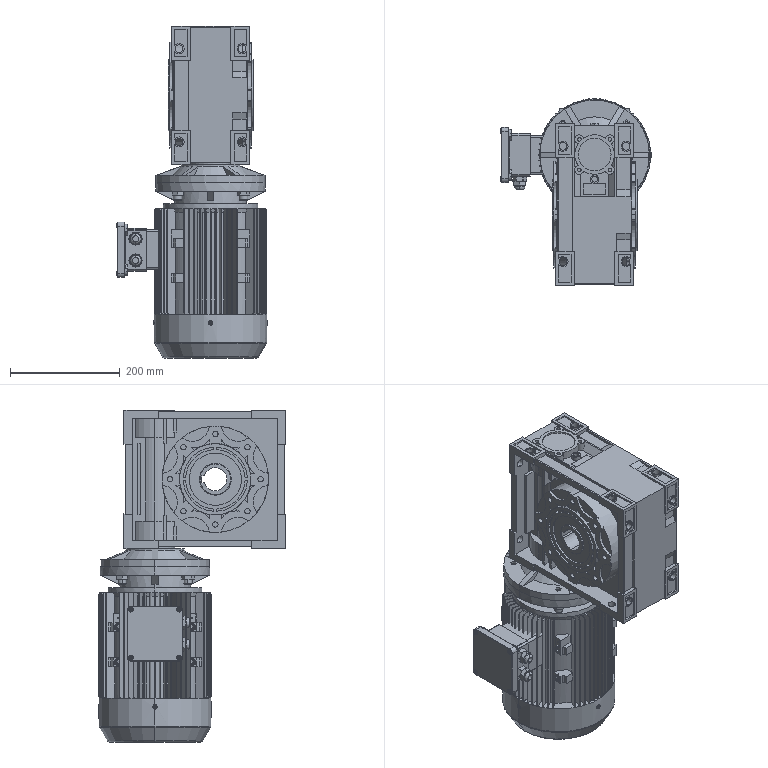Part | SolidWorks | 3 solids | 2273 faces | box 274.826 x 342.025 x 605.25 mm | volume 17102127 mm3 | plane 1389 | cylinder 687 | cone 133 | torus 64 | commonest cylinder face diameters 8.2 x112 168.1 x52 10 x48 61.845 x40 4.32 x36 18.2 x33